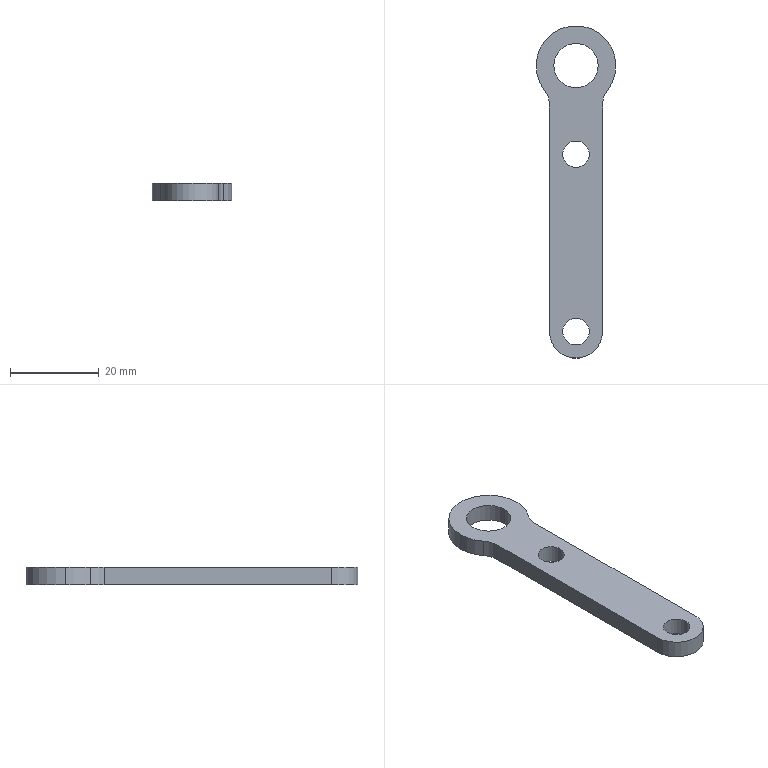Part | SolidWorks | features Extrusion 1 | 1 solid | 16 faces | box 18 x 75 x 4 mm | volume 3190 mm3 | cylinder 12 | plane 4 | commonest cylinder face diameters 6 x4 10 x4 18 x3 12 x1
STEP:
#1=CARTESIAN_POINT('',(-3.,-60.,4.));
#2=VERTEX_POINT('',#1);
#3=CARTESIAN_POINT('',(3.,-60.,4.));
#4=VERTEX_POINT('',#3);
#5=CARTESIAN_POINT('',(0.,-60.,4.));
#6=DIRECTION('',(0.,0.,1.));
#7=DIRECTION('',(1.,0.,0.));
#8=AXIS2_PLACEMENT_3D('',#5,#6,#7);
#9=CIRCLE('',#8,3.);
#10=EDGE_CURVE('',#2,#4,#9,.T.);
#11=ORIENTED_EDGE('',*,*,#10,.T.);
#12=CARTESIAN_POINT('',(3.,-60.,0.));
#13=VERTEX_POINT('',#12);
#14=CARTESIAN_POINT('',(3.,-60.,4.));
#15=DIRECTION('',(0.,0.,-1.));
#16=VECTOR('',#15,1000.);
#17=LINE('',#14,#16);
#18=EDGE_CURVE('',#4,#13,#17,.T.);
#19=ORIENTED_EDGE('',*,*,#18,.T.);
#20=CARTESIAN_POINT('',(-3.,-60.,0.));
#21=VERTEX_POINT('',#20);
#22=CARTESIAN_POINT('',(0.,-60.,0.));
#23=DIRECTION('',(0.,0.,1.));
#24=DIRECTION('',(1.,0.,0.));
#25=AXIS2_PLACEMENT_3D('',#22,#23,#24);
#26=CIRCLE('',#25,3.);
#27=EDGE_CURVE('',#21,#13,#26,.T.);
#28=ORIENTED_EDGE('',*,*,#27,.F.);
#29=CARTESIAN_POINT('',(-3.,-60.,4.));
#30=DIRECTION('',(0.,0.,-1.));
#31=VECTOR('',#30,1000.);
#32=LINE('',#29,#31);
#33=EDGE_CURVE('',#2,#21,#32,.T.);
#34=ORIENTED_EDGE('',*,*,#33,.F.);
#35=EDGE_LOOP('',(#11,#19,#28,#34));
#36=FACE_OUTER_BOUND('',#35,.T.);
#37=CARTESIAN_POINT('',(0.,-60.,4.));
#38=DIRECTION('',(0.,0.,-1.));
#39=DIRECTION('',(-1.,0.,0.));
#40=AXIS2_PLACEMENT_3D('',#37,#38,#39);
#41=CYLINDRICAL_SURFACE('',#40,3.);
#42=ADVANCED_FACE('',(#36),#41,.F.);
#43=CARTESIAN_POINT('',(-3.,-20.,4.));
#44=VERTEX_POINT('',#43);
#45=CARTESIAN_POINT('',(3.,-20.,4.));
#46=VERTEX_POINT('',#45);
#47=CARTESIAN_POINT('',(0.,-20.,4.));
#48=DIRECTION('',(0.,0.,1.));
#49=DIRECTION('',(1.,0.,0.));
#50=AXIS2_PLACEMENT_3D('',#47,#48,#49);
#51=CIRCLE('',#50,3.);
#52=EDGE_CURVE('',#44,#46,#51,.T.);
#53=ORIENTED_EDGE('',*,*,#52,.T.);
#54=CARTESIAN_POINT('',(3.,-20.,0.));
#55=VERTEX_POINT('',#54);
#56=CARTESIAN_POINT('',(3.,-20.,4.));
#57=DIRECTION('',(0.,0.,-1.));
#58=VECTOR('',#57,1000.);
#59=LINE('',#56,#58);
#60=EDGE_CURVE('',#46,#55,#59,.T.);
#61=ORIENTED_EDGE('',*,*,#60,.T.);
#62=CARTESIAN_POINT('',(-3.,-20.,0.));
#63=VERTEX_POINT('',#62);
#64=CARTESIAN_POINT('',(0.,-20.,0.));
#65=DIRECTION('',(0.,0.,1.));
#66=DIRECTION('',(1.,0.,0.));
#67=AXIS2_PLACEMENT_3D('',#64,#65,#66);
#68=CIRCLE('',#67,3.);
#69=EDGE_CURVE('',#63,#55,#68,.T.);
#70=ORIENTED_EDGE('',*,*,#69,.F.);
#71=CARTESIAN_POINT('',(-3.,-20.,4.));
#72=DIRECTION('',(0.,0.,-1.));
#73=VECTOR('',#72,1000.);
#74=LINE('',#71,#73);
#75=EDGE_CURVE('',#44,#63,#74,.T.);
#76=ORIENTED_EDGE('',*,*,#75,.F.);
#77=EDGE_LOOP('',(#53,#61,#70,#76));
#78=FACE_OUTER_BOUND('',#77,.T.);
#79=CARTESIAN_POINT('',(0.,-20.,4.));
#80=DIRECTION('',(0.,0.,-1.));
#81=DIRECTION('',(-1.,0.,0.));
#82=AXIS2_PLACEMENT_3D('',#79,#80,#81);
#83=CYLINDRICAL_SURFACE('',#82,3.);
#84=ADVANCED_FACE('',(#78),#83,.F.);
#85=CARTESIAN_POINT('',(-5.,0.,4.));
#86=VERTEX_POINT('',#85);
#87=CARTESIAN_POINT('',(5.,0.,4.));
#88=VERTEX_POINT('',#87);
#89=CARTESIAN_POINT('',(0.,0.,4.));
#90=DIRECTION('',(0.,0.,1.));
#91=DIRECTION('',(1.,0.,0.));
#92=AXIS2_PLACEMENT_3D('',#89,#90,#91);
#93=CIRCLE('',#92,5.);
#94=EDGE_CURVE('',#86,#88,#93,.T.);
#95=ORIENTED_EDGE('',*,*,#94,.T.);
#96=CARTESIAN_POINT('',(5.,0.,0.));
#97=VERTEX_POINT('',#96);
#98=CARTESIAN_POINT('',(5.,0.,4.));
#99=DIRECTION('',(0.,0.,-1.));
#100=VECTOR('',#99,1000.);
#101=LINE('',#98,#100);
#102=EDGE_CURVE('',#88,#97,#101,.T.);
#103=ORIENTED_EDGE('',*,*,#102,.T.);
#104=CARTESIAN_POINT('',(-5.,0.,0.));
#105=VERTEX_POINT('',#104);
#106=CARTESIAN_POINT('',(0.,0.,0.));
#107=DIRECTION('',(0.,0.,1.));
#108=DIRECTION('',(1.,0.,0.));
#109=AXIS2_PLACEMENT_3D('',#106,#107,#108);
#110=CIRCLE('',#109,5.);
#111=EDGE_CURVE('',#105,#97,#110,.T.);
#112=ORIENTED_EDGE('',*,*,#111,.F.);
#113=CARTESIAN_POINT('',(-5.,0.,4.));
#114=DIRECTION('',(0.,0.,-1.));
#115=VECTOR('',#114,1000.);
#116=LINE('',#113,#115);
#117=EDGE_CURVE('',#86,#105,#116,.T.);
#118=ORIENTED_EDGE('',*,*,#117,.F.);
#119=EDGE_LOOP('',(#95,#103,#112,#118));
#120=FACE_OUTER_BOUND('',#119,.T.);
#121=CARTESIAN_POINT('',(0.,0.,4.));
#122=DIRECTION('',(0.,0.,-1.));
#123=DIRECTION('',(-1.,0.,0.));
#124=AXIS2_PLACEMENT_3D('',#121,#122,#123);
#125=CYLINDRICAL_SURFACE('',#124,5.);
#126=ADVANCED_FACE('',(#120),#125,.F.);
#127=CARTESIAN_POINT('',(9.,0.,4.));
#128=VERTEX_POINT('',#127);
#129=CARTESIAN_POINT('',(-9.,0.,4.));
#130=VERTEX_POINT('',#129);
#131=CARTESIAN_POINT('',(0.,0.,4.));
#132=DIRECTION('',(0.,0.,1.));
#133=DIRECTION('',(1.,0.,0.));
#134=AXIS2_PLACEMENT_3D('',#131,#132,#133);
#135=CIRCLE('',#134,9.);
#136=EDGE_CURVE('',#128,#130,#135,.T.);
#137=ORIENTED_EDGE('',*,*,#136,.F.);
#138=CARTESIAN_POINT('',(9.,0.,0.));
#139=VERTEX_POINT('',#138);
#140=CARTESIAN_POINT('',(9.,0.,4.));
#141=DIRECTION('',(0.,0.,-1.));
#142=VECTOR('',#141,1000.);
#143=LINE('',#140,#142);
#144=EDGE_CURVE('',#128,#139,#143,.T.);
#145=ORIENTED_EDGE('',*,*,#144,.T.);
#146=CARTESIAN_POINT('',(-9.,0.,0.));
#147=VERTEX_POINT('',#146);
#148=CARTESIAN_POINT('',(0.,0.,0.));
#149=DIRECTION('',(0.,0.,1.));
#150=DIRECTION('',(1.,0.,0.));
#151=AXIS2_PLACEMENT_3D('',#148,#149,#150);
#152=CIRCLE('',#151,9.);
#153=EDGE_CURVE('',#139,#147,#152,.T.);
#154=ORIENTED_EDGE('',*,*,#153,.T.);
#155=CARTESIAN_POINT('',(-9.,0.,4.));
#156=DIRECTION('',(0.,0.,-1.));
#157=VECTOR('',#156,1000.);
#158=LINE('',#155,#157);
#159=EDGE_CURVE('',#130,#147,#158,.T.);
#160=ORIENTED_EDGE('',*,*,#159,.F.);
#161=EDGE_LOOP('',(#137,#145,#154,#160));
#162=FACE_OUTER_BOUND('',#161,.T.);
#163=CARTESIAN_POINT('',(0.,0.,4.));
#164=DIRECTION('',(0.,0.,-1.));
#165=DIRECTION('',(-1.,0.,0.));
#166=AXIS2_PLACEMENT_3D('',#163,#164,#165);
#167=CYLINDRICAL_SURFACE('',#166,9.);
#168=ADVANCED_FACE('',(#162),#167,.T.);
#169=CARTESIAN_POINT('',(-7.071,-5.567,4.));
#170=VERTEX_POINT('',#169);
#171=CARTESIAN_POINT('',(0.,0.,4.));
#172=DIRECTION('',(0.,0.,1.));
#173=DIRECTION('',(1.,0.,0.));
#174=AXIS2_PLACEMENT_3D('',#171,#172,#173);
#175=CIRCLE('',#174,9.);
#176=EDGE_CURVE('',#130,#170,#175,.T.);
#177=ORIENTED_EDGE('',*,*,#176,.F.);
#178=ORIENTED_EDGE('',*,*,#159,.T.);
#179=CARTESIAN_POINT('',(-7.071,-5.567,0.));
#180=VERTEX_POINT('',#179);
#181=CARTESIAN_POINT('',(0.,0.,0.));
#182=DIRECTION('',(0.,0.,1.));
#183=DIRECTION('',(1.,0.,0.));
#184=AXIS2_PLACEMENT_3D('',#181,#182,#183);
#185=CIRCLE('',#184,9.);
#186=EDGE_CURVE('',#147,#180,#185,.T.);
#187=ORIENTED_EDGE('',*,*,#186,.T.);
#188=CARTESIAN_POINT('',(-7.071,-5.567,4.));
#189=DIRECTION('',(0.,0.,-1.));
#190=VECTOR('',#189,1000.);
#191=LINE('',#188,#190);
#192=EDGE_CURVE('',#170,#180,#191,.T.);
#193=ORIENTED_EDGE('',*,*,#192,.F.);
#194=EDGE_LOOP('',(#177,#178,#187,#193));
#195=FACE_OUTER_BOUND('',#194,.T.);
#196=CARTESIAN_POINT('',(0.,0.,4.));
#197=DIRECTION('',(0.,0.,-1.));
#198=DIRECTION('',(-1.,0.,0.));
#199=AXIS2_PLACEMENT_3D('',#196,#197,#198);
#200=CYLINDRICAL_SURFACE('',#199,9.);
#201=ADVANCED_FACE('',(#195),#200,.T.);
#202=ORIENTED_EDGE('',*,*,#52,.F.);
#203=CARTESIAN_POINT('',(0.,-20.,4.));
#204=DIRECTION('',(0.,0.,1.));
#205=DIRECTION('',(1.,0.,0.));
#206=AXIS2_PLACEMENT_3D('',#203,#204,#205);
#207=CIRCLE('',#206,3.);
#208=EDGE_CURVE('',#46,#44,#207,.T.);
#209=ORIENTED_EDGE('',*,*,#208,.F.);
#210=EDGE_LOOP('',(#202,#209));
#211=FACE_BOUND('',#210,.T.);
#212=CARTESIAN_POINT('',(-6.,-60.,4.));
#213=VERTEX_POINT('',#212);
#214=CARTESIAN_POINT('',(6.,-60.,4.));
#215=VERTEX_POINT('',#214);
#216=CARTESIAN_POINT('',(0.,-60.,4.));
#217=DIRECTION('',(0.,0.,1.));
#218=DIRECTION('',(1.,0.,0.));
#219=AXIS2_PLACEMENT_3D('',#216,#217,#218);
#220=CIRCLE('',#219,6.);
#221=EDGE_CURVE('',#213,#215,#220,.T.);
#222=ORIENTED_EDGE('',*,*,#221,.T.);
#223=CARTESIAN_POINT('',(6.,-8.66,4.));
#224=VERTEX_POINT('',#223);
#225=CARTESIAN_POINT('',(6.,-60.,4.));
#226=DIRECTION('',(0.,1.,0.));
#227=VECTOR('',#226,1000.);
#228=LINE('',#225,#227);
#229=EDGE_CURVE('',#215,#224,#228,.T.);
#230=ORIENTED_EDGE('',*,*,#229,.T.);
#231=CARTESIAN_POINT('',(7.071,-5.567,4.));
#232=VERTEX_POINT('',#231);
#233=CARTESIAN_POINT('',(11.,-8.66,4.));
#234=DIRECTION('',(0.,0.,-1.));
#235=DIRECTION('',(1.,0.,0.));
#236=AXIS2_PLACEMENT_3D('',#233,#234,#235);
#237=CIRCLE('',#236,5.);
#238=EDGE_CURVE('',#224,#232,#237,.T.);
#239=ORIENTED_EDGE('',*,*,#238,.T.);
#240=CARTESIAN_POINT('',(0.,0.,4.));
#241=DIRECTION('',(0.,0.,1.));
#242=DIRECTION('',(1.,0.,0.));
#243=AXIS2_PLACEMENT_3D('',#240,#241,#242);
#244=CIRCLE('',#243,9.);
#245=EDGE_CURVE('',#232,#128,#244,.T.);
#246=ORIENTED_EDGE('',*,*,#245,.T.);
#247=ORIENTED_EDGE('',*,*,#136,.T.);
#248=ORIENTED_EDGE('',*,*,#176,.T.);
#249=CARTESIAN_POINT('',(-6.,-8.66,4.));
#250=VERTEX_POINT('',#249);
#251=CARTESIAN_POINT('',(-11.,-8.66,4.));
#252=DIRECTION('',(0.,0.,-1.));
#253=DIRECTION('',(1.,0.,0.));
#254=AXIS2_PLACEMENT_3D('',#251,#252,#253);
#255=CIRCLE('',#254,5.);
#256=EDGE_CURVE('',#170,#250,#255,.T.);
#257=ORIENTED_EDGE('',*,*,#256,.T.);
#258=CARTESIAN_POINT('',(-6.,-60.,4.));
#259=DIRECTION('',(0.,-1.,0.));
#260=VECTOR('',#259,1000.);
#261=LINE('',#258,#260);
#262=EDGE_CURVE('',#250,#213,#261,.T.);
#263=ORIENTED_EDGE('',*,*,#262,.T.);
#264=EDGE_LOOP('',(#222,#230,#239,#246,#247,#248,#257,#263));
#265=FACE_OUTER_BOUND('',#264,.T.);
#266=ORIENTED_EDGE('',*,*,#94,.F.);
#267=CARTESIAN_POINT('',(0.,0.,4.));
#268=DIRECTION('',(0.,0.,1.));
#269=DIRECTION('',(1.,0.,0.));
#270=AXIS2_PLACEMENT_3D('',#267,#268,#269);
#271=CIRCLE('',#270,5.);
#272=EDGE_CURVE('',#88,#86,#271,.T.);
#273=ORIENTED_EDGE('',*,*,#272,.F.);
#274=EDGE_LOOP('',(#266,#273));
#275=FACE_BOUND('',#274,.T.);
#276=ORIENTED_EDGE('',*,*,#10,.F.);
#277=CARTESIAN_POINT('',(0.,-60.,4.));
#278=DIRECTION('',(0.,0.,1.));
#279=DIRECTION('',(1.,0.,0.));
#280=AXIS2_PLACEMENT_3D('',#277,#278,#279);
#281=CIRCLE('',#280,3.);
#282=EDGE_CURVE('',#4,#2,#281,.T.);
#283=ORIENTED_EDGE('',*,*,#282,.F.);
#284=EDGE_LOOP('',(#276,#283));
#285=FACE_BOUND('',#284,.T.);
#286=CARTESIAN_POINT('',(0.,-60.,4.));
#287=DIRECTION('',(0.,0.,1.));
#288=DIRECTION('',(1.,0.,0.));
#289=AXIS2_PLACEMENT_3D('',#286,#287,#288);
#290=PLANE('',#289);
#291=ADVANCED_FACE('',(#211,#265,#275,#285),#290,.T.);
#292=ORIENTED_EDGE('',*,*,#69,.T.);
#293=CARTESIAN_POINT('',(0.,-20.,0.));
#294=DIRECTION('',(0.,0.,1.));
#295=DIRECTION('',(1.,0.,0.));
#296=AXIS2_PLACEMENT_3D('',#293,#294,#295);
#297=CIRCLE('',#296,3.);
#298=EDGE_CURVE('',#55,#63,#297,.T.);
#299=ORIENTED_EDGE('',*,*,#298,.T.);
#300=EDGE_LOOP('',(#292,#299));
#301=FACE_BOUND('',#300,.T.);
#302=CARTESIAN_POINT('',(-6.,-60.,0.));
#303=VERTEX_POINT('',#302);
#304=CARTESIAN_POINT('',(6.,-60.,0.));
#305=VERTEX_POINT('',#304);
#306=CARTESIAN_POINT('',(0.,-60.,0.));
#307=DIRECTION('',(0.,0.,1.));
#308=DIRECTION('',(1.,0.,0.));
#309=AXIS2_PLACEMENT_3D('',#306,#307,#308);
#310=CIRCLE('',#309,6.);
#311=EDGE_CURVE('',#303,#305,#310,.T.);
#312=ORIENTED_EDGE('',*,*,#311,.F.);
#313=CARTESIAN_POINT('',(-6.,-8.66,0.));
#314=VERTEX_POINT('',#313);
#315=CARTESIAN_POINT('',(-6.,-60.,0.));
#316=DIRECTION('',(0.,-1.,0.));
#317=VECTOR('',#316,1000.);
#318=LINE('',#315,#317);
#319=EDGE_CURVE('',#314,#303,#318,.T.);
#320=ORIENTED_EDGE('',*,*,#319,.F.);
#321=CARTESIAN_POINT('',(-11.,-8.66,0.));
#322=DIRECTION('',(0.,0.,-1.));
#323=DIRECTION('',(1.,0.,0.));
#324=AXIS2_PLACEMENT_3D('',#321,#322,#323);
#325=CIRCLE('',#324,5.);
#326=EDGE_CURVE('',#180,#314,#325,.T.);
#327=ORIENTED_EDGE('',*,*,#326,.F.);
#328=ORIENTED_EDGE('',*,*,#186,.F.);
#329=ORIENTED_EDGE('',*,*,#153,.F.);
#330=CARTESIAN_POINT('',(7.071,-5.567,0.));
#331=VERTEX_POINT('',#330);
#332=CARTESIAN_POINT('',(0.,0.,0.));
#333=DIRECTION('',(0.,0.,1.));
#334=DIRECTION('',(1.,0.,0.));
#335=AXIS2_PLACEMENT_3D('',#332,#333,#334);
#336=CIRCLE('',#335,9.);
#337=EDGE_CURVE('',#331,#139,#336,.T.);
#338=ORIENTED_EDGE('',*,*,#337,.F.);
#339=CARTESIAN_POINT('',(6.,-8.66,0.));
#340=VERTEX_POINT('',#339);
#341=CARTESIAN_POINT('',(11.,-8.66,0.));
#342=DIRECTION('',(0.,0.,-1.));
#343=DIRECTION('',(1.,0.,0.));
#344=AXIS2_PLACEMENT_3D('',#341,#342,#343);
#345=CIRCLE('',#344,5.);
#346=EDGE_CURVE('',#340,#331,#345,.T.);
#347=ORIENTED_EDGE('',*,*,#346,.F.);
#348=CARTESIAN_POINT('',(6.,-60.,0.));
#349=DIRECTION('',(0.,1.,0.));
#350=VECTOR('',#349,1000.);
#351=LINE('',#348,#350);
#352=EDGE_CURVE('',#305,#340,#351,.T.);
#353=ORIENTED_EDGE('',*,*,#352,.F.);
#354=EDGE_LOOP('',(#312,#320,#327,#328,#329,#338,#347,#353));
#355=FACE_OUTER_BOUND('',#354,.T.);
#356=ORIENTED_EDGE('',*,*,#111,.T.);
#357=CARTESIAN_POINT('',(0.,0.,0.));
#358=DIRECTION('',(0.,0.,1.));
#359=DIRECTION('',(1.,0.,0.));
#360=AXIS2_PLACEMENT_3D('',#357,#358,#359);
#361=CIRCLE('',#360,5.);
#362=EDGE_CURVE('',#97,#105,#361,.T.);
#363=ORIENTED_EDGE('',*,*,#362,.T.);
#364=EDGE_LOOP('',(#356,#363));
#365=FACE_BOUND('',#364,.T.);
#366=ORIENTED_EDGE('',*,*,#27,.T.);
#367=CARTESIAN_POINT('',(0.,-60.,0.));
#368=DIRECTION('',(0.,0.,1.));
#369=DIRECTION('',(1.,0.,0.));
#370=AXIS2_PLACEMENT_3D('',#367,#368,#369);
#371=CIRCLE('',#370,3.);
#372=EDGE_CURVE('',#13,#21,#371,.T.);
#373=ORIENTED_EDGE('',*,*,#372,.T.);
#374=EDGE_LOOP('',(#366,#373));
#375=FACE_BOUND('',#374,.T.);
#376=CARTESIAN_POINT('',(0.,-60.,0.));
#377=DIRECTION('',(0.,0.,1.));
#378=DIRECTION('',(1.,0.,0.));
#379=AXIS2_PLACEMENT_3D('',#376,#377,#378);
#380=PLANE('',#379);
#381=ADVANCED_FACE('',(#301,#355,#365,#375),#380,.F.);
#382=ORIENTED_EDGE('',*,*,#311,.T.);
#383=CARTESIAN_POINT('',(6.,-60.,4.));
#384=DIRECTION('',(0.,0.,-1.));
#385=VECTOR('',#384,1000.);
#386=LINE('',#383,#385);
#387=EDGE_CURVE('',#215,#305,#386,.T.);
#388=ORIENTED_EDGE('',*,*,#387,.F.);
#389=ORIENTED_EDGE('',*,*,#221,.F.);
#390=CARTESIAN_POINT('',(-6.,-60.,4.));
#391=DIRECTION('',(0.,0.,-1.));
#392=VECTOR('',#391,1000.);
#393=LINE('',#390,#392);
#394=EDGE_CURVE('',#213,#303,#393,.T.);
#395=ORIENTED_EDGE('',*,*,#394,.T.);
#396=EDGE_LOOP('',(#382,#388,#389,#395));
#397=FACE_OUTER_BOUND('',#396,.T.);
#398=CARTESIAN_POINT('',(0.,-60.,4.));
#399=DIRECTION('',(0.,0.,-1.));
#400=DIRECTION('',(-1.,0.,0.));
#401=AXIS2_PLACEMENT_3D('',#398,#399,#400);
#402=CYLINDRICAL_SURFACE('',#401,6.);
#403=ADVANCED_FACE('',(#397),#402,.T.);
#404=ORIENTED_EDGE('',*,*,#352,.T.);
#405=CARTESIAN_POINT('',(6.,-8.66,4.));
#406=DIRECTION('',(0.,0.,-1.));
#407=VECTOR('',#406,1000.);
#408=LINE('',#405,#407);
#409=EDGE_CURVE('',#224,#340,#408,.T.);
#410=ORIENTED_EDGE('',*,*,#409,.F.);
#411=ORIENTED_EDGE('',*,*,#229,.F.);
#412=ORIENTED_EDGE('',*,*,#387,.T.);
#413=EDGE_LOOP('',(#404,#410,#411,#412));
#414=FACE_OUTER_BOUND('',#413,.T.);
#415=CARTESIAN_POINT('',(6.,-60.,4.));
#416=DIRECTION('',(-1.,0.,0.));
#417=DIRECTION('',(0.,0.,1.));
#418=AXIS2_PLACEMENT_3D('',#415,#416,#417);
#419=PLANE('',#418);
#420=ADVANCED_FACE('',(#414),#419,.F.);
#421=ORIENTED_EDGE('',*,*,#346,.T.);
#422=CARTESIAN_POINT('',(7.071,-5.567,4.));
#423=DIRECTION('',(0.,0.,-1.));
#424=VECTOR('',#423,1000.);
#425=LINE('',#422,#424);
#426=EDGE_CURVE('',#232,#331,#425,.T.);
#427=ORIENTED_EDGE('',*,*,#426,.F.);
#428=ORIENTED_EDGE('',*,*,#238,.F.);
#429=ORIENTED_EDGE('',*,*,#409,.T.);
#430=EDGE_LOOP('',(#421,#427,#428,#429));
#431=FACE_OUTER_BOUND('',#430,.T.);
#432=CARTESIAN_POINT('',(11.,-8.66,4.));
#433=DIRECTION('',(0.,0.,-1.));
#434=DIRECTION('',(-1.,0.,0.));
#435=AXIS2_PLACEMENT_3D('',#432,#433,#434);
#436=CYLINDRICAL_SURFACE('',#435,5.);
#437=ADVANCED_FACE('',(#431),#436,.F.);
#438=ORIENTED_EDGE('',*,*,#144,.F.);
#439=ORIENTED_EDGE('',*,*,#245,.F.);
#440=ORIENTED_EDGE('',*,*,#426,.T.);
#441=ORIENTED_EDGE('',*,*,#337,.T.);
#442=EDGE_LOOP('',(#438,#439,#440,#441));
#443=FACE_OUTER_BOUND('',#442,.T.);
#444=CARTESIAN_POINT('',(0.,0.,4.));
#445=DIRECTION('',(0.,0.,-1.));
#446=DIRECTION('',(-1.,0.,0.));
#447=AXIS2_PLACEMENT_3D('',#444,#445,#446);
#448=CYLINDRICAL_SURFACE('',#447,9.);
#449=ADVANCED_FACE('',(#443),#448,.T.);
#450=ORIENTED_EDGE('',*,*,#326,.T.);
#451=CARTESIAN_POINT('',(-6.,-8.66,4.));
#452=DIRECTION('',(0.,0.,-1.));
#453=VECTOR('',#452,1000.);
#454=LINE('',#451,#453);
#455=EDGE_CURVE('',#250,#314,#454,.T.);
#456=ORIENTED_EDGE('',*,*,#455,.F.);
#457=ORIENTED_EDGE('',*,*,#256,.F.);
#458=ORIENTED_EDGE('',*,*,#192,.T.);
#459=EDGE_LOOP('',(#450,#456,#457,#458));
#460=FACE_OUTER_BOUND('',#459,.T.);
#461=CARTESIAN_POINT('',(-11.,-8.66,4.));
#462=DIRECTION('',(0.,0.,-1.));
#463=DIRECTION('',(-1.,0.,0.));
#464=AXIS2_PLACEMENT_3D('',#461,#462,#463);
#465=CYLINDRICAL_SURFACE('',#464,5.);
#466=ADVANCED_FACE('',(#460),#465,.F.);
#467=ORIENTED_EDGE('',*,*,#319,.T.);
#468=ORIENTED_EDGE('',*,*,#394,.F.);
#469=ORIENTED_EDGE('',*,*,#262,.F.);
#470=ORIENTED_EDGE('',*,*,#455,.T.);
#471=EDGE_LOOP('',(#467,#468,#469,#470));
#472=FACE_OUTER_BOUND('',#471,.T.);
#473=CARTESIAN_POINT('',(-6.,-60.,4.));
#474=DIRECTION('',(1.,0.,0.));
#475=DIRECTION('',(0.,0.,-1.));
#476=AXIS2_PLACEMENT_3D('',#473,#474,#475);
#477=PLANE('',#476);
#478=ADVANCED_FACE('',(#472),#477,.F.);
#479=ORIENTED_EDGE('',*,*,#102,.F.);
#480=ORIENTED_EDGE('',*,*,#272,.T.);
#481=ORIENTED_EDGE('',*,*,#117,.T.);
#482=ORIENTED_EDGE('',*,*,#362,.F.);
#483=EDGE_LOOP('',(#479,#480,#481,#482));
#484=FACE_OUTER_BOUND('',#483,.T.);
#485=CARTESIAN_POINT('',(0.,0.,4.));
#486=DIRECTION('',(0.,0.,-1.));
#487=DIRECTION('',(-1.,0.,0.));
#488=AXIS2_PLACEMENT_3D('',#485,#486,#487);
#489=CYLINDRICAL_SURFACE('',#488,5.);
#490=ADVANCED_FACE('',(#484),#489,.F.);
#491=ORIENTED_EDGE('',*,*,#60,.F.);
#492=ORIENTED_EDGE('',*,*,#208,.T.);
#493=ORIENTED_EDGE('',*,*,#75,.T.);
#494=ORIENTED_EDGE('',*,*,#298,.F.);
#495=EDGE_LOOP('',(#491,#492,#493,#494));
#496=FACE_OUTER_BOUND('',#495,.T.);
#497=CARTESIAN_POINT('',(0.,-20.,4.));
#498=DIRECTION('',(0.,0.,-1.));
#499=DIRECTION('',(-1.,0.,0.));
#500=AXIS2_PLACEMENT_3D('',#497,#498,#499);
#501=CYLINDRICAL_SURFACE('',#500,3.);
#502=ADVANCED_FACE('',(#496),#501,.F.);
#503=ORIENTED_EDGE('',*,*,#18,.F.);
#504=ORIENTED_EDGE('',*,*,#282,.T.);
#505=ORIENTED_EDGE('',*,*,#33,.T.);
#506=ORIENTED_EDGE('',*,*,#372,.F.);
#507=EDGE_LOOP('',(#503,#504,#505,#506));
#508=FACE_OUTER_BOUND('',#507,.T.);
#509=CARTESIAN_POINT('',(0.,-60.,4.));
#510=DIRECTION('',(0.,0.,-1.));
#511=DIRECTION('',(-1.,0.,0.));
#512=AXIS2_PLACEMENT_3D('',#509,#510,#511);
#513=CYLINDRICAL_SURFACE('',#512,3.);
#514=ADVANCED_FACE('',(#508),#513,.F.);
#515=CLOSED_SHELL('',(#42,#84,#126,#168,#201,#291,#381,#403,#420,#437,#449,#466,#478,#490,#502,#514));
#516=MANIFOLD_SOLID_BREP('',#515);
#517=CARTESIAN_POINT('',(0.,0.,0.));
#518=DIRECTION('',(0.,0.,1.));
#519=DIRECTION('',(1.,0.,0.));
#520=AXIS2_PLACEMENT_3D('',#517,#518,#519);
#521=(LENGTH_UNIT()NAMED_UNIT(*)SI_UNIT(.MILLI.,.METRE.));
#522=UNCERTAINTY_MEASURE_WITH_UNIT(LENGTH_MEASURE(0.00001),#521,'','');
#523=(NAMED_UNIT(*)PLANE_ANGLE_UNIT()SI_UNIT($,.RADIAN.));
#524=(NAMED_UNIT(*)SI_UNIT($,.STERADIAN.)SOLID_ANGLE_UNIT());
#525=(GEOMETRIC_REPRESENTATION_CONTEXT(3)GLOBAL_UNCERTAINTY_ASSIGNED_CONTEXT((#522))GLOBAL_UNIT_ASSIGNED_CONTEXT((#521,#523,#524))REPRESENTATION_CONTEXT('',''));
#526=ADVANCED_BREP_SHAPE_REPRESENTATION('',(#516,#520),#525);